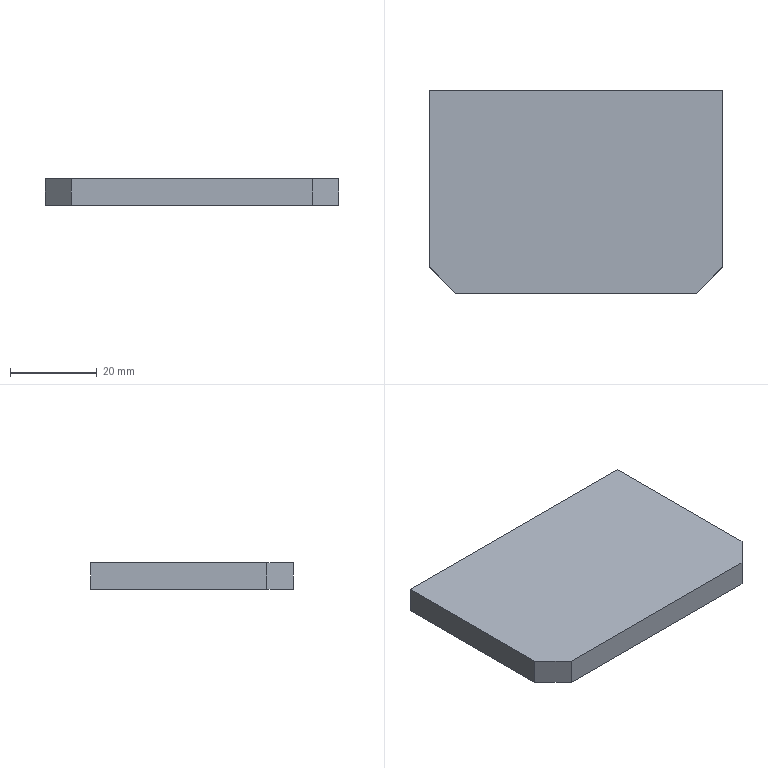Part | STEP file | SYL_0392D6J1SYL0380DJ10-1680959 | 1 solid | 8 faces | box 67.5 x 46.5 x 6 mm | volume 18616 mm3 | plane 8
STEP:
#1=CARTESIAN_POINT('',(33.75,23.25,6.));
#2=VERTEX_POINT('',#1);
#3=CARTESIAN_POINT('',(33.75,-17.25,6.));
#4=VERTEX_POINT('',#3);
#5=CARTESIAN_POINT('',(33.75,23.25,6.));
#6=DIRECTION('',(0.,-1.,0.));
#7=VECTOR('',#6,1000.);
#8=LINE('',#5,#7);
#9=EDGE_CURVE('',#2,#4,#8,.T.);
#10=ORIENTED_EDGE('',*,*,#9,.T.);
#11=CARTESIAN_POINT('',(33.75,-17.25,0.));
#12=VERTEX_POINT('',#11);
#13=CARTESIAN_POINT('',(33.75,-17.25,6.));
#14=DIRECTION('',(0.,0.,-1.));
#15=VECTOR('',#14,1000.);
#16=LINE('',#13,#15);
#17=EDGE_CURVE('',#4,#12,#16,.T.);
#18=ORIENTED_EDGE('',*,*,#17,.T.);
#19=CARTESIAN_POINT('',(33.75,23.25,0.));
#20=VERTEX_POINT('',#19);
#21=CARTESIAN_POINT('',(33.75,23.25,0.));
#22=DIRECTION('',(0.,-1.,0.));
#23=VECTOR('',#22,1000.);
#24=LINE('',#21,#23);
#25=EDGE_CURVE('',#20,#12,#24,.T.);
#26=ORIENTED_EDGE('',*,*,#25,.F.);
#27=CARTESIAN_POINT('',(33.75,23.25,6.));
#28=DIRECTION('',(0.,0.,-1.));
#29=VECTOR('',#28,1000.);
#30=LINE('',#27,#29);
#31=EDGE_CURVE('',#2,#20,#30,.T.);
#32=ORIENTED_EDGE('',*,*,#31,.F.);
#33=EDGE_LOOP('',(#10,#18,#26,#32));
#34=FACE_OUTER_BOUND('',#33,.T.);
#35=CARTESIAN_POINT('',(33.75,0.,3.));
#36=DIRECTION('',(-1.,0.,0.));
#37=DIRECTION('',(0.,0.,1.));
#38=AXIS2_PLACEMENT_3D('',#35,#36,#37);
#39=PLANE('',#38);
#40=ADVANCED_FACE('',(#34),#39,.F.);
#41=CARTESIAN_POINT('',(27.75,-23.25,0.));
#42=VERTEX_POINT('',#41);
#43=CARTESIAN_POINT('',(33.75,-17.25,0.));
#44=DIRECTION('',(-0.7071,-0.7071,0.));
#45=VECTOR('',#44,1000.);
#46=LINE('',#43,#45);
#47=EDGE_CURVE('',#12,#42,#46,.T.);
#48=ORIENTED_EDGE('',*,*,#47,.F.);
#49=ORIENTED_EDGE('',*,*,#17,.F.);
#50=CARTESIAN_POINT('',(27.75,-23.25,6.));
#51=VERTEX_POINT('',#50);
#52=CARTESIAN_POINT('',(27.75,-23.25,6.));
#53=DIRECTION('',(0.7071,0.7071,0.));
#54=VECTOR('',#53,1000.);
#55=LINE('',#52,#54);
#56=EDGE_CURVE('',#51,#4,#55,.T.);
#57=ORIENTED_EDGE('',*,*,#56,.F.);
#58=CARTESIAN_POINT('',(27.75,-23.25,0.));
#59=DIRECTION('',(0.,0.,1.));
#60=VECTOR('',#59,1000.);
#61=LINE('',#58,#60);
#62=EDGE_CURVE('',#42,#51,#61,.T.);
#63=ORIENTED_EDGE('',*,*,#62,.F.);
#64=EDGE_LOOP('',(#48,#49,#57,#63));
#65=FACE_OUTER_BOUND('',#64,.T.);
#66=CARTESIAN_POINT('',(30.75,-20.25,3.));
#67=DIRECTION('',(0.7071,-0.7071,0.));
#68=DIRECTION('',(0.,0.,-1.));
#69=AXIS2_PLACEMENT_3D('',#66,#67,#68);
#70=PLANE('',#69);
#71=ADVANCED_FACE('',(#65),#70,.T.);
#72=CARTESIAN_POINT('',(-27.75,-23.25,0.));
#73=VERTEX_POINT('',#72);
#74=CARTESIAN_POINT('',(27.75,-23.25,0.));
#75=DIRECTION('',(-1.,0.,0.));
#76=VECTOR('',#75,1000.);
#77=LINE('',#74,#76);
#78=EDGE_CURVE('',#42,#73,#77,.T.);
#79=ORIENTED_EDGE('',*,*,#78,.F.);
#80=ORIENTED_EDGE('',*,*,#62,.T.);
#81=CARTESIAN_POINT('',(-27.75,-23.25,6.));
#82=VERTEX_POINT('',#81);
#83=CARTESIAN_POINT('',(27.75,-23.25,6.));
#84=DIRECTION('',(-1.,0.,0.));
#85=VECTOR('',#84,1000.);
#86=LINE('',#83,#85);
#87=EDGE_CURVE('',#51,#82,#86,.T.);
#88=ORIENTED_EDGE('',*,*,#87,.T.);
#89=CARTESIAN_POINT('',(-27.75,-23.25,6.));
#90=DIRECTION('',(0.,0.,-1.));
#91=VECTOR('',#90,1000.);
#92=LINE('',#89,#91);
#93=EDGE_CURVE('',#82,#73,#92,.T.);
#94=ORIENTED_EDGE('',*,*,#93,.T.);
#95=EDGE_LOOP('',(#79,#80,#88,#94));
#96=FACE_OUTER_BOUND('',#95,.T.);
#97=CARTESIAN_POINT('',(0.,-23.25,3.));
#98=DIRECTION('',(0.,1.,0.));
#99=DIRECTION('',(1.,0.,0.));
#100=AXIS2_PLACEMENT_3D('',#97,#98,#99);
#101=PLANE('',#100);
#102=ADVANCED_FACE('',(#96),#101,.F.);
#103=ORIENTED_EDGE('',*,*,#56,.T.);
#104=ORIENTED_EDGE('',*,*,#9,.F.);
#105=CARTESIAN_POINT('',(-33.75,23.25,6.));
#106=VERTEX_POINT('',#105);
#107=CARTESIAN_POINT('',(-33.75,23.25,6.));
#108=DIRECTION('',(1.,0.,0.));
#109=VECTOR('',#108,1000.);
#110=LINE('',#107,#109);
#111=EDGE_CURVE('',#106,#2,#110,.T.);
#112=ORIENTED_EDGE('',*,*,#111,.F.);
#113=CARTESIAN_POINT('',(-33.75,-17.25,6.));
#114=VERTEX_POINT('',#113);
#115=CARTESIAN_POINT('',(-33.75,-17.25,6.));
#116=DIRECTION('',(0.,1.,0.));
#117=VECTOR('',#116,1000.);
#118=LINE('',#115,#117);
#119=EDGE_CURVE('',#114,#106,#118,.T.);
#120=ORIENTED_EDGE('',*,*,#119,.F.);
#121=CARTESIAN_POINT('',(-33.75,-17.25,6.));
#122=DIRECTION('',(0.7071,-0.7071,0.));
#123=VECTOR('',#122,1000.);
#124=LINE('',#121,#123);
#125=EDGE_CURVE('',#114,#82,#124,.T.);
#126=ORIENTED_EDGE('',*,*,#125,.T.);
#127=ORIENTED_EDGE('',*,*,#87,.F.);
#128=EDGE_LOOP('',(#103,#104,#112,#120,#126,#127));
#129=FACE_OUTER_BOUND('',#128,.T.);
#130=CARTESIAN_POINT('',(0.,0.,6.));
#131=DIRECTION('',(0.,0.,1.));
#132=DIRECTION('',(1.,0.,0.));
#133=AXIS2_PLACEMENT_3D('',#130,#131,#132);
#134=PLANE('',#133);
#135=ADVANCED_FACE('',(#129),#134,.T.);
#136=ORIENTED_EDGE('',*,*,#31,.T.);
#137=CARTESIAN_POINT('',(-33.75,23.25,0.));
#138=VERTEX_POINT('',#137);
#139=CARTESIAN_POINT('',(-33.75,23.25,0.));
#140=DIRECTION('',(1.,0.,0.));
#141=VECTOR('',#140,1000.);
#142=LINE('',#139,#141);
#143=EDGE_CURVE('',#138,#20,#142,.T.);
#144=ORIENTED_EDGE('',*,*,#143,.F.);
#145=CARTESIAN_POINT('',(-33.75,23.25,6.));
#146=DIRECTION('',(0.,0.,-1.));
#147=VECTOR('',#146,1000.);
#148=LINE('',#145,#147);
#149=EDGE_CURVE('',#106,#138,#148,.T.);
#150=ORIENTED_EDGE('',*,*,#149,.F.);
#151=ORIENTED_EDGE('',*,*,#111,.T.);
#152=EDGE_LOOP('',(#136,#144,#150,#151));
#153=FACE_OUTER_BOUND('',#152,.T.);
#154=CARTESIAN_POINT('',(0.,23.25,3.));
#155=DIRECTION('',(0.,-1.,0.));
#156=DIRECTION('',(0.,0.,-1.));
#157=AXIS2_PLACEMENT_3D('',#154,#155,#156);
#158=PLANE('',#157);
#159=ADVANCED_FACE('',(#153),#158,.F.);
#160=CARTESIAN_POINT('',(-33.75,-17.25,0.));
#161=VERTEX_POINT('',#160);
#162=CARTESIAN_POINT('',(-33.75,-17.25,0.));
#163=DIRECTION('',(0.,1.,0.));
#164=VECTOR('',#163,1000.);
#165=LINE('',#162,#164);
#166=EDGE_CURVE('',#161,#138,#165,.T.);
#167=ORIENTED_EDGE('',*,*,#166,.F.);
#168=CARTESIAN_POINT('',(-33.75,-17.25,0.));
#169=DIRECTION('',(0.,0.,1.));
#170=VECTOR('',#169,1000.);
#171=LINE('',#168,#170);
#172=EDGE_CURVE('',#161,#114,#171,.T.);
#173=ORIENTED_EDGE('',*,*,#172,.T.);
#174=ORIENTED_EDGE('',*,*,#119,.T.);
#175=ORIENTED_EDGE('',*,*,#149,.T.);
#176=EDGE_LOOP('',(#167,#173,#174,#175));
#177=FACE_OUTER_BOUND('',#176,.T.);
#178=CARTESIAN_POINT('',(-33.75,0.,3.));
#179=DIRECTION('',(1.,0.,0.));
#180=DIRECTION('',(0.,1.,0.));
#181=AXIS2_PLACEMENT_3D('',#178,#179,#180);
#182=PLANE('',#181);
#183=ADVANCED_FACE('',(#177),#182,.F.);
#184=CARTESIAN_POINT('',(-27.75,-23.25,0.));
#185=DIRECTION('',(-0.7071,0.7071,0.));
#186=VECTOR('',#185,1000.);
#187=LINE('',#184,#186);
#188=EDGE_CURVE('',#73,#161,#187,.T.);
#189=ORIENTED_EDGE('',*,*,#188,.F.);
#190=ORIENTED_EDGE('',*,*,#93,.F.);
#191=ORIENTED_EDGE('',*,*,#125,.F.);
#192=ORIENTED_EDGE('',*,*,#172,.F.);
#193=EDGE_LOOP('',(#189,#190,#191,#192));
#194=FACE_OUTER_BOUND('',#193,.T.);
#195=CARTESIAN_POINT('',(-30.75,-20.25,3.));
#196=DIRECTION('',(-0.7071,-0.7071,0.));
#197=DIRECTION('',(-0.7071,0.7071,0.));
#198=AXIS2_PLACEMENT_3D('',#195,#196,#197);
#199=PLANE('',#198);
#200=ADVANCED_FACE('',(#194),#199,.T.);
#201=ORIENTED_EDGE('',*,*,#166,.T.);
#202=ORIENTED_EDGE('',*,*,#143,.T.);
#203=ORIENTED_EDGE('',*,*,#25,.T.);
#204=ORIENTED_EDGE('',*,*,#47,.T.);
#205=ORIENTED_EDGE('',*,*,#78,.T.);
#206=ORIENTED_EDGE('',*,*,#188,.T.);
#207=EDGE_LOOP('',(#201,#202,#203,#204,#205,#206));
#208=FACE_OUTER_BOUND('',#207,.T.);
#209=CARTESIAN_POINT('',(0.,0.,0.));
#210=DIRECTION('',(0.,0.,1.));
#211=DIRECTION('',(1.,0.,0.));
#212=AXIS2_PLACEMENT_3D('',#209,#210,#211);
#213=PLANE('',#212);
#214=ADVANCED_FACE('',(#208),#213,.F.);
#215=CLOSED_SHELL('',(#40,#71,#102,#135,#159,#183,#200,#214));
#216=MANIFOLD_SOLID_BREP('',#215);
#217=CARTESIAN_POINT('',(0.,0.,0.));
#218=DIRECTION('',(0.,0.,1.));
#219=DIRECTION('',(1.,0.,0.));
#220=AXIS2_PLACEMENT_3D('',#217,#218,#219);
#221=(LENGTH_UNIT()NAMED_UNIT(*)SI_UNIT(.MILLI.,.METRE.));
#222=UNCERTAINTY_MEASURE_WITH_UNIT(LENGTH_MEASURE(0.00001),#221,'','');
#223=(NAMED_UNIT(*)PLANE_ANGLE_UNIT()SI_UNIT($,.RADIAN.));
#224=(NAMED_UNIT(*)SI_UNIT($,.STERADIAN.)SOLID_ANGLE_UNIT());
#225=(GEOMETRIC_REPRESENTATION_CONTEXT(3)GLOBAL_UNCERTAINTY_ASSIGNED_CONTEXT((#222))GLOBAL_UNIT_ASSIGNED_CONTEXT((#221,#223,#224))REPRESENTATION_CONTEXT('',''));
#226=ADVANCED_BREP_SHAPE_REPRESENTATION('',(#216,#220),#225);